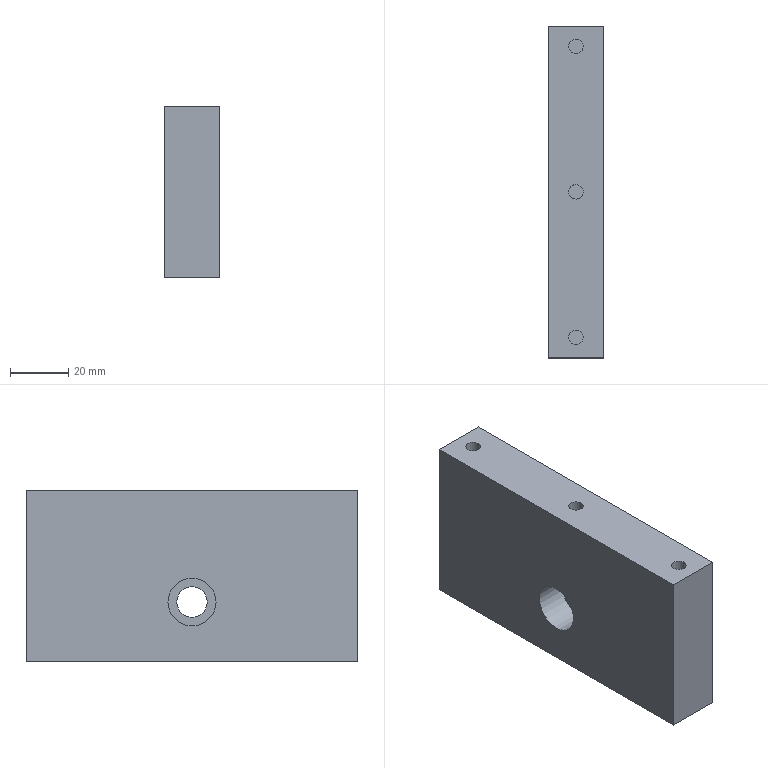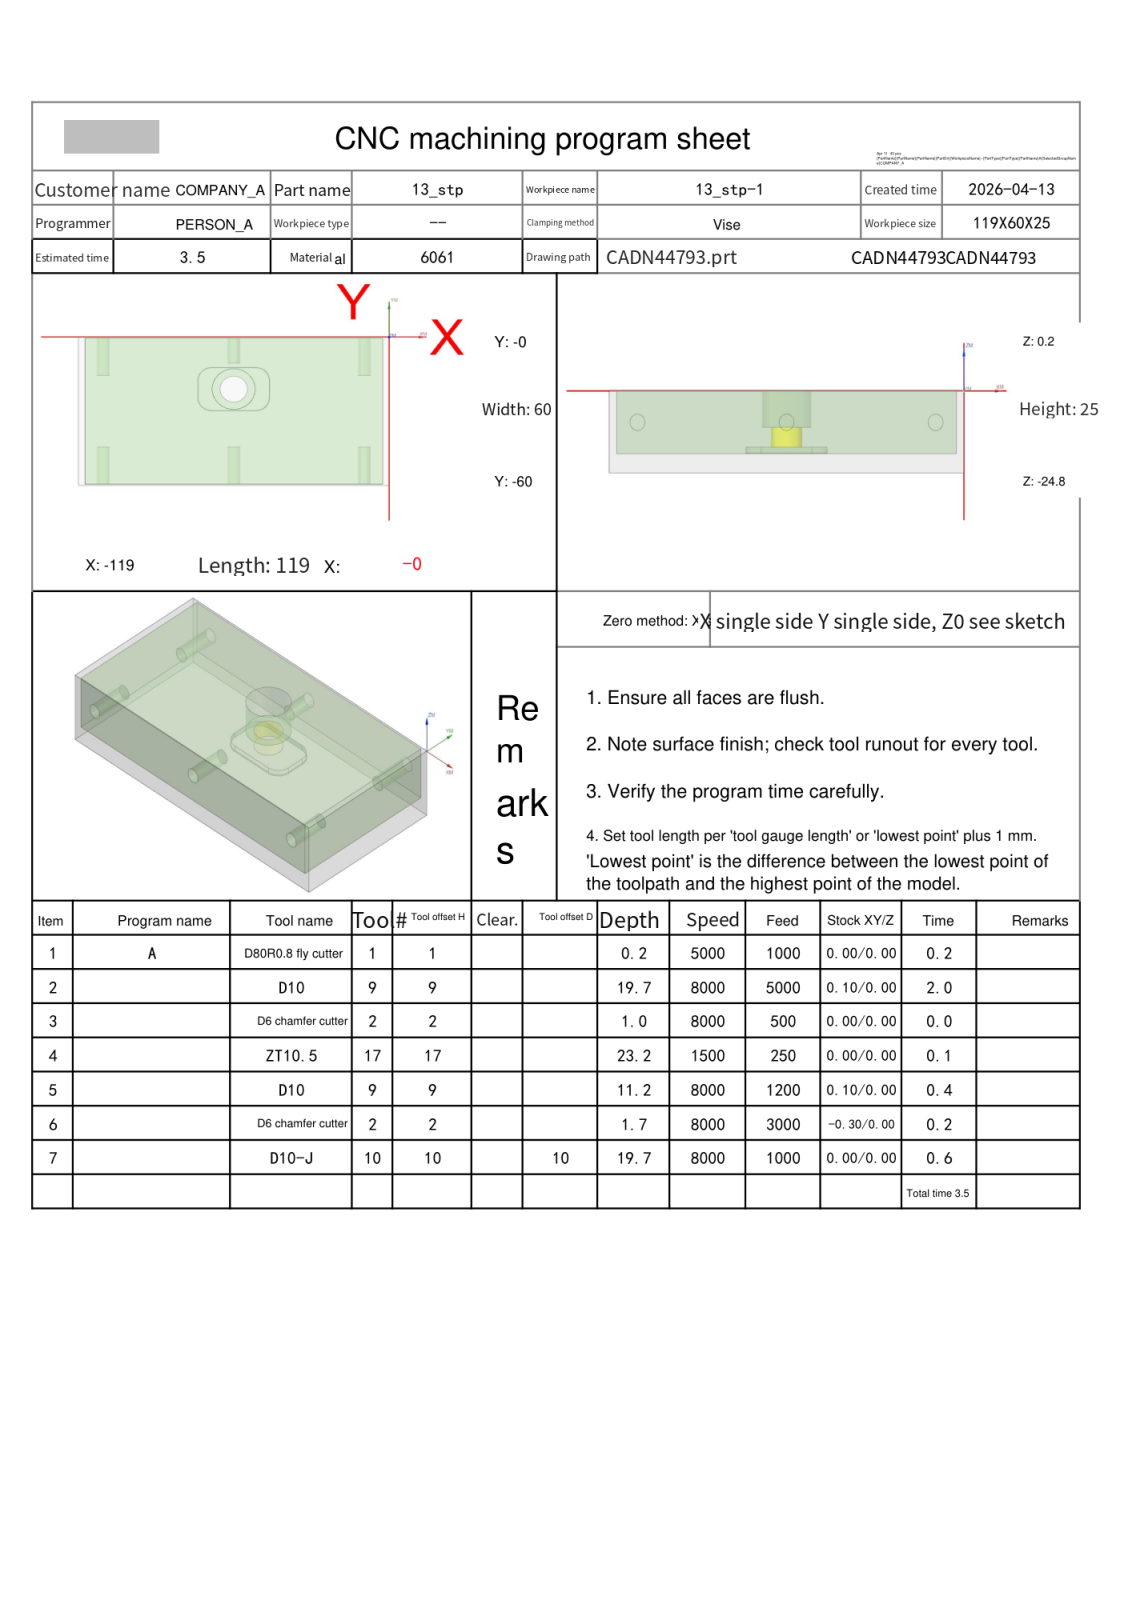NC program | NX | posted by the shop | part box 19 x 114 x 59 mm
Whole program:
%
O0001
(Machine time: 4.89 MIN)
(===Total Tool:5===)
(T1=D80R0.8 fly cutter D=80.  R=0.8  D- H01 Z=0.    )
(T9=D10     D=10.  R=0.   D-  H09 Z=-19.5 )
(T2=D6 chamfer cutter   D=6.   R=0.   D- H02 Z=-1.5  )
(T17=ZT10.5 D=10.5 DR_a=118 D-  H17 Z=-23.  )
(T10=D10-J  D=10.  R=0.   D10 H10 Z=-19.5 )
G80 G90 G17 G49 G40
G91 G28 Z0
M01
N1 T01 M06
(D80R0.8 fly cutter  D=80. R=0.8 H=01 ce=0.00 di=0.00)
G00 G90 G54 X-161.5 Y-30. M03 S5000
G43 H01 Z20.
M08
Z2.
G01 Z0.0 F1000.
X-156.5
X37.5
X42.5
Z2.
G00 Z20.
G91 G28 Z0.0
M05
M09
G91 G28 Z0.0
M01
N2 T09 M06
(D10  D=10. R=0. H=09 ce=0.10 di=0.00)
G00 G90 G54 X-59.5 Y-64.6 M03 S8000
G43 H09 Z20.
M08
Z.5
G01 X-116.5 Z.379 F5000.
G02 X-121.6 Y-59.5 Z.362 I0.0 J5.1
G01 Y-.5 Z.238
G02 X-116.5 Y4.6 Z.221 I5.1 J0.0
G01 X-2.5 Z-.021
G02 X2.6 Y-.5 Z-.038 I0.0 J-5.1
G01 Y-59.5 Z-.162
G02 X-2.5 Y-64.6 Z-.179 I-5.1 J0.0
G01 X-116.5 Z-.421
G02 X-121.6 Y-59.5 Z-.438 I0.0 J5.1
G01 Y-.5 Z-.562
G02 X-116.5 Y4.6 Z-.579 I5.1 J0.0
G01 X-2.5 Z-.821
G02 X2.6 Y-.5 Z-.838 I0.0 J-5.1
G01 Y-59.5 Z-.962
G02 X-2.5 Y-64.6 Z-.979 I-5.1 J0.0
G01 X-116.5 Z-1.221
G02 X-121.6 Y-59.5 Z-1.238 I0.0 J5.1
G01 Y-.5 Z-1.362
G02 X-116.5 Y4.6 Z-1.379 I5.1 J0.0
G01 X-2.5 Z-1.621
G02 X2.6 Y-.5 Z-1.638 I0.0 J-5.1
G01 Y-59.5 Z-1.762
G02 X-2.5 Y-64.6 Z-1.779 I-5.1 J0.0
G01 X-116.5 Z-2.021
G02 X-121.6 Y-59.5 Z-2.038 I0.0 J5.1
G01 Y-.5 Z-2.162
G02 X-116.5 Y4.6 Z-2.179 I5.1 J0.0
G01 X-2.5 Z-2.421
G02 X2.6 Y-.5 Z-2.438 I0.0 J-5.1
G01 Y-59.5 Z-2.562
G02 X-2.5 Y-64.6 Z-2.579 I-5.1 J0.0
G01 X-116.5 Z-2.821
G02 X-121.6 Y-59.5 Z-2.838 I0.0 J5.1
G01 Y-.5 Z-2.962
G02 X-116.5 Y4.6 Z-2.979 I5.1 J0.0
G01 X-2.5 Z-3.221
G02 X2.6 Y-.5 Z-3.238 I0.0 J-5.1
G01 Y-59.5 Z-3.362
G02 X-2.5 Y-64.6 Z-3.379 I-5.1 J0.0
G01 X-116.5 Z-3.621
G02 X-121.6 Y-59.5 Z-3.638 I0.0 J5.1
G01 Y-.5 Z-3.762
G02 X-116.5 Y4.6 Z-3.779 I5.1 J0.0
G01 X-2.5 Z-4.021
G02 X2.6 Y-.5 Z-4.038 I0.0 J-5.1
G01 Y-59.5 Z-4.162
G02 X-2.5 Y-64.6 Z-4.179 I-5.1 J0.0
G01 X-116.5 Z-4.421
G02 X-121.6 Y-59.5 Z-4.438 I0.0 J5.1
G01 Y-.5 Z-4.562
G02 X-116.5 Y4.6 Z-4.579 I5.1 J0.0
G01 X-2.5 Z-4.821
G02 X2.6 Y-.5 Z-4.838 I0.0 J-5.1
G01 Y-59.5 Z-4.962
G02 X-2.5 Y-64.6 Z-4.979 I-5.1 J0.0
G01 X-116.5 Z-5.221
G02 X-121.6 Y-59.5 Z-5.238 I0.0 J5.1
G01 Y-.5 Z-5.362
G02 X-116.5 Y4.6 Z-5.379 I5.1 J0.0
G01 X-2.5 Z-5.621
G02 X2.6 Y-.5 Z-5.638 I0.0 J-5.1
G01 Y-59.5 Z-5.762
G02 X-2.5 Y-64.6 Z-5.779 I-5.1 J0.0
G01 X-116.5 Z-6.021
G02 X-121.6 Y-59.5 Z-6.038 I0.0 J5.1
G01 Y-.5 Z-6.162
G02 X-116.5 Y4.6 Z-6.179 I5.1 J0.0
G01 X-2.5 Z-6.421
G02 X2.6 Y-.5 Z-6.438 I0.0 J-5.1
G01 Y-59.5 Z-6.562
G02 X-2.5 Y-64.6 Z-6.579 I-5.1 J0.0
G01 X-116.5 Z-6.821
G02 X-121.6 Y-59.5 Z-6.838 I0.0 J5.1
G01 Y-.5 Z-6.962
G02 X-116.5 Y4.6 Z-6.979 I5.1 J0.0
G01 X-2.5 Z-7.221
G02 X2.6 Y-.5 Z-7.238 I0.0 J-5.1
G01 Y-59.5 Z-7.362
G02 X-2.5 Y-64.6 Z-7.379 I-5.1 J0.0
G01 X-116.5 Z-7.621
G02 X-121.6 Y-59.5 Z-7.638 I0.0 J5.1
G01 Y-.5 Z-7.762
G02 X-116.5 Y4.6 Z-7.779 I5.1 J0.0
G01 X-2.5 Z-8.021
G02 X2.6 Y-.5 Z-8.038 I0.0 J-5.1
G01 Y-59.5 Z-8.162
G02 X-2.5 Y-64.6 Z-8.179 I-5.1 J0.0
G01 X-116.5 Z-8.421
G02 X-121.6 Y-59.5 Z-8.438 I0.0 J5.1
G01 Y-.5 Z-8.562
G02 X-116.5 Y4.6 Z-8.579 I5.1 J0.0
G01 X-2.5 Z-8.821
G02 X2.6 Y-.5 Z-8.838 I0.0 J-5.1
G01 Y-59.5 Z-8.962
G02 X-2.5 Y-64.6 Z-8.979 I-5.1 J0.0
G01 X-116.5 Z-9.221
G02 X-121.6 Y-59.5 Z-9.238 I0.0 J5.1
G01 Y-.5 Z-9.362
G02 X-116.5 Y4.6 Z-9.379 I5.1 J0.0
G01 X-2.5 Z-9.621
G02 X2.6 Y-.5 Z-9.638 I0.0 J-5.1
G01 Y-59.5 Z-9.762
G02 X-2.5 Y-64.6 Z-9.779 I-5.1 J0.0
G01 X-116.5 Z-10.021
G02 X-121.6 Y-59.5 Z-10.038 I0.0 J5.1
G01 Y-.5 Z-10.162
G02 X-116.5 Y4.6 Z-10.179 I5.1 J0.0
G01 X-2.5 Z-10.421
G02 X2.6 Y-.5 Z-10.438 I0.0 J-5.1
G01 Y-59.5 Z-10.562
G02 X-2.5 Y-64.6 Z-10.579 I-5.1 J0.0
G01 X-116.5 Z-10.821
G02 X-121.6 Y-59.5 Z-10.838 I0.0 J5.1
G01 Y-.5 Z-10.962
G02 X-116.5 Y4.6 Z-10.979 I5.1 J0.0
G01 X-2.5 Z-11.221
G02 X2.6 Y-.5 Z-11.238 I0.0 J-5.1
G01 Y-59.5 Z-11.362
G02 X-2.5 Y-64.6 Z-11.379 I-5.1 J0.0
G01 X-116.5 Z-11.621
G02 X-121.6 Y-59.5 Z-11.638 I0.0 J5.1
G01 Y-.5 Z-11.762
G02 X-116.5 Y4.6 Z-11.779 I5.1 J0.0
G01 X-2.5 Z-12.021
G02 X2.6 Y-.5 Z-12.038 I0.0 J-5.1
G01 Y-59.5 Z-12.162
G02 X-2.5 Y-64.6 Z-12.179 I-5.1 J0.0
G01 X-116.5 Z-12.421
G02 X-121.6 Y-59.5 Z-12.438 I0.0 J5.1
G01 Y-.5 Z-12.562
G02 X-116.5 Y4.6 Z-12.579 I5.1 J0.0
G01 X-2.5 Z-12.821
G02 X2.6 Y-.5 Z-12.838 I0.0 J-5.1
G01 Y-59.5 Z-12.962
G02 X-2.5 Y-64.6 Z-12.979 I-5.1 J0.0
G01 X-116.5 Z-13.221
G02 X-121.6 Y-59.5 Z-13.238 I0.0 J5.1
G01 Y-.5 Z-13.362
G02 X-116.5 Y4.6 Z-13.379 I5.1 J0.0
G01 X-2.5 Z-13.621
G02 X2.6 Y-.5 Z-13.638 I0.0 J-5.1
G01 Y-59.5 Z-13.762
G02 X-2.5 Y-64.6 Z-13.779 I-5.1 J0.0
G01 X-116.5 Z-14.021
G02 X-121.6 Y-59.5 Z-14.038 I0.0 J5.1
G01 Y-.5 Z-14.162
G02 X-116.5 Y4.6 Z-14.179 I5.1 J0.0
G01 X-2.5 Z-14.421
G02 X2.6 Y-.5 Z-14.438 I0.0 J-5.1
G01 Y-59.5 Z-14.562
G02 X-2.5 Y-64.6 Z-14.579 I-5.1 J0.0
G01 X-116.5 Z-14.821
G02 X-121.6 Y-59.5 Z-14.838 I0.0 J5.1
G01 Y-.5 Z-14.962
G02 X-116.5 Y4.6 Z-14.979 I5.1 J0.0
G01 X-2.5 Z-15.221
G02 X2.6 Y-.5 Z-15.238 I0.0 J-5.1
G01 Y-59.5 Z-15.362
G02 X-2.5 Y-64.6 Z-15.379 I-5.1 J0.0
G01 X-116.5 Z-15.621
G02 X-121.6 Y-59.5 Z-15.638 I0.0 J5.1
G01 Y-.5 Z-15.762
G02 X-116.5 Y4.6 Z-15.779 I5.1 J0.0
G01 X-2.5 Z-16.021
G02 X2.6 Y-.5 Z-16.038 I0.0 J-5.1
G01 Y-59.5 Z-16.162
G02 X-2.5 Y-64.6 Z-16.179 I-5.1 J0.0
G01 X-116.5 Z-16.421
G02 X-121.6 Y-59.5 Z-16.438 I0.0 J5.1
G01 Y-.5 Z-16.562
G02 X-116.5 Y4.6 Z-16.579 I5.1 J0.0
G01 X-2.5 Z-16.821
G02 X2.6 Y-.5 Z-16.838 I0.0 J-5.1
G01 Y-59.5 Z-16.962
G02 X-2.5 Y-64.6 Z-16.979 I-5.1 J0.0
G01 X-116.5 Z-17.221
G02 X-121.6 Y-59.5 Z-17.238 I0.0 J5.1
G01 Y-.5 Z-17.362
G02 X-116.5 Y4.6 Z-17.379 I5.1 J0.0
G01 X-2.5 Z-17.621
G02 X2.6 Y-.5 Z-17.638 I0.0 J-5.1
G01 Y-59.5 Z-17.762
G02 X-2.5 Y-64.6 Z-17.779 I-5.1 J0.0
G01 X-116.5 Z-18.021
G02 X-121.6 Y-59.5 Z-18.038 I0.0 J5.1
G01 Y-.5 Z-18.162
G02 X-116.5 Y4.6 Z-18.179 I5.1 J0.0
G01 X-2.5 Z-18.421
G02 X2.6 Y-.5 Z-18.438 I0.0 J-5.1
G01 Y-59.5 Z-18.562
G02 X-2.5 Y-64.6 Z-18.579 I-5.1 J0.0
G01 X-116.5 Z-18.821
G02 X-121.6 Y-59.5 Z-18.838 I0.0 J5.1
G01 Y-.5 Z-18.962
G02 X-116.5 Y4.6 Z-18.979 I5.1 J0.0
G01 X-2.5 Z-19.221
G02 X2.6 Y-.5 Z-19.238 I0.0 J-5.1
G01 Y-59.5 Z-19.362
G02 X-2.5 Y-64.6 Z-19.379 I-5.1 J0.0
G01 X-59.5 Z-19.5
X-116.5
G02 X-121.6 Y-59.5 I0.0 J5.1
G01 Y-.5
G02 X-116.5 Y4.6 I5.1 J0.0
G01 X-2.5
G02 X2.6 Y-.5 I0.0 J-5.1
G01 Y-59.5
G02 X-2.5 Y-64.6 I-5.1 J0.0
G01 X-59.5
X-60.
Z-18.5
G00 Z20.
G91 G28 Z0.0
M05
M09
G91 G28 Z0.0
M01
N3 T02 M06
(D6 chamfer cutter  D=6. R=0. H=02 ce=0.00 di=0.00)
G00 G90 G54 X-59.5 Y-21.05 M03 S8000
G43 H02 Z20.
M08
G98 G81 X-59.5 Y-21.05 Z-.8 R1. F500.
G80
G00 Z20.
G91 G28 Z0.0
M05
M09
G91 G28 Z0.0
M01
N4 T17 M06
(ZT10.5 D=10.5 DR_a=118 H=17)
G00 G90 G54 X-59.5 Y-21.05 M03 S1500
G43 H17 Z20.
M08
G98 G83 X-59.5 Y-21.05 Z-23. R1. F250. Q2.
G80
G00 Z20.
G91 G28 Z0.0
M05
M09
G91 G28 Z0.0
M01
N5 T09 M06
(D10  D=10. R=0. H=09 ce=0.10 di=0.00)
G00 G90 G54 X-59.5 Y-21.05 M03 S8000
G43 H09 Z20.
M08
Z.5
G03 X-57.925 Y-22.625 I1.575 J0.0 F1200.
X-56.35 Y-21.05 I0.0 J1.575
X-56.35 Y-21.05 Z0.0 I-3.15 J0.0
X-56.35 Y-21.05 Z-.5 I-3.15 J0.0
X-56.35 Y-21.05 Z-1. I-3.15 J0.0
X-56.35 Y-21.05 Z-1.5 I-3.15 J0.0
X-56.35 Y-21.05 Z-2. I-3.15 J0.0
X-56.35 Y-21.05 Z-2.5 I-3.15 J0.0
X-56.35 Y-21.05 Z-3. I-3.15 J0.0
X-56.35 Y-21.05 Z-3.5 I-3.15 J0.0
X-56.35 Y-21.05 Z-4. I-3.15 J0.0
X-56.35 Y-21.05 Z-4.5 I-3.15 J0.0
X-56.35 Y-21.05 Z-5. I-3.15 J0.0
X-56.35 Y-21.05 Z-5.5 I-3.15 J0.0
X-56.35 Y-21.05 Z-6. I-3.15 J0.0
X-56.35 Y-21.05 Z-6.5 I-3.15 J0.0
X-56.35 Y-21.05 Z-7. I-3.15 J0.0
X-56.35 Y-21.05 Z-7.5 I-3.15 J0.0
X-56.35 Y-21.05 Z-8. I-3.15 J0.0
X-56.35 Y-21.05 Z-8.5 I-3.15 J0.0
X-56.35 Y-21.05 Z-9. I-3.15 J0.0
X-56.35 Y-21.05 Z-9.5 I-3.15 J0.0
X-56.35 Y-21.05 Z-10. I-3.15 J0.0
X-56.35 Y-21.05 Z-10.5 I-3.15 J0.0
X-56.35 Y-21.05 Z-11. I-3.15 J0.0
X-59.5 Y-17.9 I-3.15 J0.0
X-62.65 Y-21.05 I0.0 J-3.15
X-59.5 Y-24.2 I3.15 J0.0
X-56.35 Y-21.05 I0.0 J3.15
X-57.925 Y-19.475 I-1.575 J0.0
X-59.5 Y-21.05 I0.0 J-1.575
G00 Z20.
G91 G28 Z0.0
M05
M09
G91 G28 Z0.0
M01
N6 T02 M06
(D6 chamfer cutter  D=6. R=0. H=02 ce=0.00 di=0.00)
G00 G90 G54 X-59.75 Y1.628 M03 S8000
G43 H02 Z20.
M08
Z2.099
G01 Z-1.499 F3000.
G03 X-59.83 Y1.328 I.52 J-.3
X-59.53 Y.808 I.6 J0.0
G01 X-59.5 Y.8
X-2.5
G02 X-1.2 Y-.5 I0.0 J-1.3
G01 Y-59.5
G02 X-2.5 Y-60.8 I-1.3 J0.0
G01 X-116.5
G02 X-117.8 Y-59.5 I0.0 J1.3
G01 Y-.5
G02 X-116.5 Y.8 I1.3 J0.0
G01 X-59.5
X-59.47 Y.808
G03 X-59.17 Y1.328 I-.3 J.52
X-59.25 Y1.628 I-.6 J0.0
G01 Z2.099
G00 Z20.
X-59.207 Y-14.913
Z2.131
G01 Z-1.499
G03 X-59.142 Y-14.641 I-.535 J.272
X-59.47 Y-14.106 I-.6 J0.0
G01 X-59.5 Y-14.1
G03 X-66.45 Y-21.05 I0.0 J-6.95
X-59.5 Y-28. I6.95 J0.0
X-52.55 Y-21.05 I0.0 J6.95
X-59.5 Y-14.1 I-6.95 J0.0
G01 X-59.53 Y-14.106
G03 X-59.858 Y-14.641 I.272 J-.535
X-59.793 Y-14.913 I.6 J0.0
G01 Z2.131
G00 Z20.
G00 G90 X-66.719 Y-23.262 M03 S8000
Z20.
Z2.5
G01 X-66.55 Y-23.759 Z2.309 F800.
X-66.317 Y-24.303 Z2.094
X-66.041 Y-24.827 Z1.878
X-65.725 Y-25.327 Z1.663
X-65.371 Y-25.801 Z1.447
X-64.981 Y-26.247 Z1.232
X-64.557 Y-26.66 Z1.016
X-64.103 Y-27.039 Z.801
X-63.62 Y-27.381 Z.585
X-63.111 Y-27.684 Z.37
X-62.581 Y-27.946 Z.155
X-62.031 Y-28.166 Z-.061
X-61.466 Y-28.343 Z-.276
X-60.889 Y-28.474 Z-.492
X-60.303 Y-28.56 Z-.707
X-59.713 Y-28.6 Z-.923
X-59.5 Z-1.
G03 X-51.95 Y-21.05 I0.0 J7.55
X-59.5 Y-13.5 I-7.55 J0.0
X-67.05 Y-21.05 I0.0 J-7.55
X-59.5 Y-28.6 I7.55 J0.0
X-59. Y-28.583 I0.0 J7.55
G01 Z1.5
G00 Z20.
G91 G28 Z0.0
M05
M09
G91 G28 Z0.0
M01
N7 T10 M06
(D10-J  D=10. R=0. H=10 ce=0.00 di=0.00)
G00 G90 G54 X-59.5 Y-21.05 M03 S8000
G43 H10 Z20.
M08
Z.5
G41 D10
G01 X-59.475 Y-21.248 F500.
G03 X-57.869 Y-22.669 I1.607 J.198
X-56.25 Y-21.05 I0.0 J1.619
X-56.25 Y-21.05 Z-4.5 I-3.25 J0.0
X-56.25 Y-21.05 Z-9.5 I-3.25 J0.0
X-60.504 Y-17.959 Z-11. I-3.25 J0.0
X-62.75 Y-21.05 I1.004 J-3.091
X-59.5 Y-24.3 I3.25 J0.0
X-56.25 Y-21.05 I0.0 J3.25
X-59.5 Y-17.8 I-3.25 J0.0
X-60.504 Y-17.959 I0.0 J-3.25
X-61.623 Y-19.499 I.5 J-1.54
X-60.004 Y-21.118 I1.619 J0.0
X-59.696 Y-21.088 I0.0 J1.619
G01 G40 X-59.5 Y-21.05
G00 Z20.
G00 G90 X-117.513 Y5.616 M03 S8000
Z20.
Z-19.
G01 Z-19.5 F1000.
G41 D10
X-117.497 Y5.417
G03 X-116.5 Y4.5 I.997 J.083
G01 X-2.5
G02 X2.5 Y-.5 I0.0 J-5.
G01 Y-59.5
G02 X-2.5 Y-64.5 I-5. J0.0
G01 X-116.5
G02 X-121.5 Y-59.5 I0.0 J5.
G01 Y-.5
G02 X-116.5 Y4.5 I5. J0.0
G01 X-116.
G03 X-115. Y5.5 I0.0 J1.
G01 G40 Y5.7
Z-19.
G00 Z20.
M05
M09
G91 G28 Z0.0
G91 G28 Y0.0
M30
%